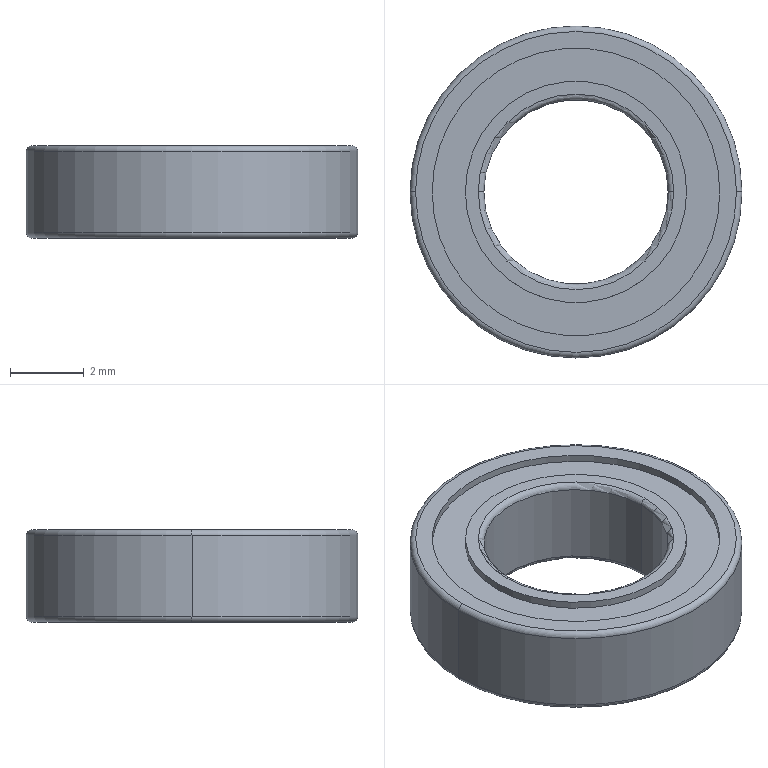Part | NX | features BREP 1 | 1 solid | 26 faces | box 9 x 9 x 2.5 mm | volume 101.727 mm3 | cylinder 12 | torus 8 | plane 6 | commonest cylinder face diameters 6 x4 7.8 x4 5 x2 9 x2
STEP:
#1=CARTESIAN_POINT('',(-4.35,0.,1.25));
#2=VERTEX_POINT('',#1);
#3=CARTESIAN_POINT('',(-4.5,0.,1.1));
#4=VERTEX_POINT('',#3);
#5=CARTESIAN_POINT('',(-4.35,0.,1.1));
#6=DIRECTION('',(0.,1.,0.));
#7=DIRECTION('',(-1.,0.,0.));
#8=AXIS2_PLACEMENT_3D('',#5,#6,#7);
#9=CIRCLE('',#8,0.15);
#10=EDGE_CURVE('',#2,#4,#9,.F.);
#11=ORIENTED_EDGE('',*,*,#10,.T.);
#12=CARTESIAN_POINT('',(4.5,0.,1.1));
#13=VERTEX_POINT('',#12);
#14=CARTESIAN_POINT('',(0.,0.,1.1));
#15=DIRECTION('',(0.,0.,-1.));
#16=DIRECTION('',(1.,0.,0.));
#17=AXIS2_PLACEMENT_3D('',#14,#15,#16);
#18=CIRCLE('',#17,4.5);
#19=EDGE_CURVE('',#13,#4,#18,.T.);
#20=ORIENTED_EDGE('',*,*,#19,.F.);
#21=CARTESIAN_POINT('',(4.35,0.,1.25));
#22=VERTEX_POINT('',#21);
#23=CARTESIAN_POINT('',(4.35,0.,1.1));
#24=DIRECTION('',(0.,-1.,0.));
#25=DIRECTION('',(0.,0.,-1.));
#26=AXIS2_PLACEMENT_3D('',#23,#24,#25);
#27=CIRCLE('',#26,0.15);
#28=EDGE_CURVE('',#22,#13,#27,.F.);
#29=ORIENTED_EDGE('',*,*,#28,.F.);
#30=CARTESIAN_POINT('',(0.,0.,1.25));
#31=DIRECTION('',(0.,0.,1.));
#32=DIRECTION('',(1.,0.,0.));
#33=AXIS2_PLACEMENT_3D('',#30,#31,#32);
#34=CIRCLE('',#33,4.35);
#35=EDGE_CURVE('',#2,#22,#34,.T.);
#36=ORIENTED_EDGE('',*,*,#35,.F.);
#37=EDGE_LOOP('',(#11,#20,#29,#36));
#38=FACE_BOUND('',#37,.T.);
#39=CARTESIAN_POINT('',(0.,0.,1.1));
#40=DIRECTION('',(0.,0.,1.));
#41=DIRECTION('',(1.,0.,0.));
#42=AXIS2_PLACEMENT_3D('',#39,#40,#41);
#43=TOROIDAL_SURFACE('',#42,4.35,0.15);
#44=ADVANCED_FACE('',(#38),#43,.T.);
#45=CARTESIAN_POINT('',(-4.5,0.,-1.1));
#46=VERTEX_POINT('',#45);
#47=CARTESIAN_POINT('',(-4.35,0.,-1.25));
#48=VERTEX_POINT('',#47);
#49=CARTESIAN_POINT('',(-4.35,0.,-1.1));
#50=DIRECTION('',(0.,1.,0.));
#51=DIRECTION('',(-1.,0.,0.));
#52=AXIS2_PLACEMENT_3D('',#49,#50,#51);
#53=CIRCLE('',#52,0.15);
#54=EDGE_CURVE('',#46,#48,#53,.F.);
#55=ORIENTED_EDGE('',*,*,#54,.T.);
#56=CARTESIAN_POINT('',(4.35,0.,-1.25));
#57=VERTEX_POINT('',#56);
#58=CARTESIAN_POINT('',(0.,0.,-1.25));
#59=DIRECTION('',(0.,0.,-1.));
#60=DIRECTION('',(1.,0.,0.));
#61=AXIS2_PLACEMENT_3D('',#58,#59,#60);
#62=CIRCLE('',#61,4.35);
#63=EDGE_CURVE('',#57,#48,#62,.T.);
#64=ORIENTED_EDGE('',*,*,#63,.F.);
#65=CARTESIAN_POINT('',(4.5,0.,-1.1));
#66=VERTEX_POINT('',#65);
#67=CARTESIAN_POINT('',(4.35,0.,-1.1));
#68=DIRECTION('',(0.,-1.,0.));
#69=DIRECTION('',(0.,0.,-1.));
#70=AXIS2_PLACEMENT_3D('',#67,#68,#69);
#71=CIRCLE('',#70,0.15);
#72=EDGE_CURVE('',#66,#57,#71,.F.);
#73=ORIENTED_EDGE('',*,*,#72,.F.);
#74=CARTESIAN_POINT('',(0.,0.,-1.1));
#75=DIRECTION('',(0.,0.,1.));
#76=DIRECTION('',(1.,0.,0.));
#77=AXIS2_PLACEMENT_3D('',#74,#75,#76);
#78=CIRCLE('',#77,4.5);
#79=EDGE_CURVE('',#46,#66,#78,.T.);
#80=ORIENTED_EDGE('',*,*,#79,.F.);
#81=EDGE_LOOP('',(#55,#64,#73,#80));
#82=FACE_BOUND('',#81,.T.);
#83=CARTESIAN_POINT('',(0.,0.,-1.1));
#84=DIRECTION('',(0.,0.,1.));
#85=DIRECTION('',(1.,0.,0.));
#86=AXIS2_PLACEMENT_3D('',#83,#84,#85);
#87=TOROIDAL_SURFACE('',#86,4.35,0.15);
#88=ADVANCED_FACE('',(#82),#87,.T.);
#89=CARTESIAN_POINT('',(-2.5,0.,1.1));
#90=VERTEX_POINT('',#89);
#91=CARTESIAN_POINT('',(-2.65,0.,1.25));
#92=VERTEX_POINT('',#91);
#93=CARTESIAN_POINT('',(-2.65,0.,1.1));
#94=DIRECTION('',(0.,1.,0.));
#95=DIRECTION('',(-1.,0.,0.));
#96=AXIS2_PLACEMENT_3D('',#93,#94,#95);
#97=CIRCLE('',#96,0.15);
#98=EDGE_CURVE('',#90,#92,#97,.F.);
#99=ORIENTED_EDGE('',*,*,#98,.T.);
#100=CARTESIAN_POINT('',(2.65,0.,1.25));
#101=VERTEX_POINT('',#100);
#102=CARTESIAN_POINT('',(0.,0.,1.25));
#103=DIRECTION('',(0.,0.,-1.));
#104=DIRECTION('',(1.,0.,0.));
#105=AXIS2_PLACEMENT_3D('',#102,#103,#104);
#106=CIRCLE('',#105,2.65);
#107=EDGE_CURVE('',#101,#92,#106,.T.);
#108=ORIENTED_EDGE('',*,*,#107,.F.);
#109=CARTESIAN_POINT('',(2.5,0.,1.1));
#110=VERTEX_POINT('',#109);
#111=CARTESIAN_POINT('',(2.65,0.,1.1));
#112=DIRECTION('',(0.,-1.,0.));
#113=DIRECTION('',(0.,0.,-1.));
#114=AXIS2_PLACEMENT_3D('',#111,#112,#113);
#115=CIRCLE('',#114,0.15);
#116=EDGE_CURVE('',#110,#101,#115,.F.);
#117=ORIENTED_EDGE('',*,*,#116,.F.);
#118=CARTESIAN_POINT('',(0.,0.,1.1));
#119=DIRECTION('',(0.,0.,1.));
#120=DIRECTION('',(1.,0.,0.));
#121=AXIS2_PLACEMENT_3D('',#118,#119,#120);
#122=CIRCLE('',#121,2.5);
#123=EDGE_CURVE('',#90,#110,#122,.T.);
#124=ORIENTED_EDGE('',*,*,#123,.F.);
#125=EDGE_LOOP('',(#99,#108,#117,#124));
#126=FACE_BOUND('',#125,.T.);
#127=CARTESIAN_POINT('',(0.,0.,1.1));
#128=DIRECTION('',(0.,0.,1.));
#129=DIRECTION('',(1.,0.,0.));
#130=AXIS2_PLACEMENT_3D('',#127,#128,#129);
#131=TOROIDAL_SURFACE('',#130,2.65,0.15);
#132=ADVANCED_FACE('',(#126),#131,.T.);
#133=CARTESIAN_POINT('',(-2.65,0.,-1.25));
#134=VERTEX_POINT('',#133);
#135=CARTESIAN_POINT('',(-2.5,0.,-1.1));
#136=VERTEX_POINT('',#135);
#137=CARTESIAN_POINT('',(-2.65,0.,-1.1));
#138=DIRECTION('',(0.,1.,0.));
#139=DIRECTION('',(-1.,0.,0.));
#140=AXIS2_PLACEMENT_3D('',#137,#138,#139);
#141=CIRCLE('',#140,0.15);
#142=EDGE_CURVE('',#134,#136,#141,.F.);
#143=ORIENTED_EDGE('',*,*,#142,.T.);
#144=CARTESIAN_POINT('',(2.5,0.,-1.1));
#145=VERTEX_POINT('',#144);
#146=CARTESIAN_POINT('',(0.,0.,-1.1));
#147=DIRECTION('',(0.,0.,-1.));
#148=DIRECTION('',(1.,0.,0.));
#149=AXIS2_PLACEMENT_3D('',#146,#147,#148);
#150=CIRCLE('',#149,2.5);
#151=EDGE_CURVE('',#145,#136,#150,.T.);
#152=ORIENTED_EDGE('',*,*,#151,.F.);
#153=CARTESIAN_POINT('',(2.65,0.,-1.25));
#154=VERTEX_POINT('',#153);
#155=CARTESIAN_POINT('',(2.65,0.,-1.1));
#156=DIRECTION('',(0.,-1.,0.));
#157=DIRECTION('',(0.,0.,-1.));
#158=AXIS2_PLACEMENT_3D('',#155,#156,#157);
#159=CIRCLE('',#158,0.15);
#160=EDGE_CURVE('',#154,#145,#159,.F.);
#161=ORIENTED_EDGE('',*,*,#160,.F.);
#162=CARTESIAN_POINT('',(0.,0.,-1.25));
#163=DIRECTION('',(0.,0.,1.));
#164=DIRECTION('',(1.,0.,0.));
#165=AXIS2_PLACEMENT_3D('',#162,#163,#164);
#166=CIRCLE('',#165,2.65);
#167=EDGE_CURVE('',#134,#154,#166,.T.);
#168=ORIENTED_EDGE('',*,*,#167,.F.);
#169=EDGE_LOOP('',(#143,#152,#161,#168));
#170=FACE_BOUND('',#169,.T.);
#171=CARTESIAN_POINT('',(0.,0.,-1.1));
#172=DIRECTION('',(0.,0.,1.));
#173=DIRECTION('',(1.,0.,0.));
#174=AXIS2_PLACEMENT_3D('',#171,#172,#173);
#175=TOROIDAL_SURFACE('',#174,2.65,0.15);
#176=ADVANCED_FACE('',(#170),#175,.T.);
#177=CARTESIAN_POINT('',(3.,0.,-1.05));
#178=VERTEX_POINT('',#177);
#179=CARTESIAN_POINT('',(3.,0.,-1.25));
#180=VERTEX_POINT('',#179);
#181=CARTESIAN_POINT('',(3.,0.,-1.05));
#182=DIRECTION('',(0.,0.,-1.));
#183=VECTOR('',#182,1000.);
#184=LINE('',#181,#183);
#185=EDGE_CURVE('',#178,#180,#184,.T.);
#186=ORIENTED_EDGE('',*,*,#185,.F.);
#187=CARTESIAN_POINT('',(-3.,0.,-1.05));
#188=VERTEX_POINT('',#187);
#189=CARTESIAN_POINT('',(0.,0.,-1.05));
#190=DIRECTION('',(0.,0.,1.));
#191=DIRECTION('',(1.,0.,0.));
#192=AXIS2_PLACEMENT_3D('',#189,#190,#191);
#193=CIRCLE('',#192,3.);
#194=EDGE_CURVE('',#188,#178,#193,.T.);
#195=ORIENTED_EDGE('',*,*,#194,.F.);
#196=CARTESIAN_POINT('',(-3.,0.,-1.25));
#197=VERTEX_POINT('',#196);
#198=CARTESIAN_POINT('',(-3.,0.,-1.05));
#199=DIRECTION('',(0.,0.,-1.));
#200=VECTOR('',#199,1000.);
#201=LINE('',#198,#200);
#202=EDGE_CURVE('',#188,#197,#201,.T.);
#203=ORIENTED_EDGE('',*,*,#202,.T.);
#204=CARTESIAN_POINT('',(0.,0.,-1.25));
#205=DIRECTION('',(0.,0.,1.));
#206=DIRECTION('',(1.,0.,0.));
#207=AXIS2_PLACEMENT_3D('',#204,#205,#206);
#208=CIRCLE('',#207,3.);
#209=EDGE_CURVE('',#197,#180,#208,.T.);
#210=ORIENTED_EDGE('',*,*,#209,.T.);
#211=EDGE_LOOP('',(#186,#195,#203,#210));
#212=FACE_BOUND('',#211,.T.);
#213=CARTESIAN_POINT('',(0.,0.,-1.05));
#214=DIRECTION('',(0.,0.,-1.));
#215=DIRECTION('',(-1.,0.,0.));
#216=AXIS2_PLACEMENT_3D('',#213,#214,#215);
#217=CYLINDRICAL_SURFACE('',#216,3.);
#218=ADVANCED_FACE('',(#212),#217,.T.);
#219=CARTESIAN_POINT('',(3.9,0.,-1.05));
#220=VERTEX_POINT('',#219);
#221=CARTESIAN_POINT('',(3.9,0.,-1.25));
#222=VERTEX_POINT('',#221);
#223=CARTESIAN_POINT('',(3.9,0.,-1.05));
#224=DIRECTION('',(0.,0.,-1.));
#225=VECTOR('',#224,1000.);
#226=LINE('',#223,#225);
#227=EDGE_CURVE('',#220,#222,#226,.T.);
#228=ORIENTED_EDGE('',*,*,#227,.F.);
#229=CARTESIAN_POINT('',(-3.9,0.,-1.05));
#230=VERTEX_POINT('',#229);
#231=CARTESIAN_POINT('',(0.,0.,-1.05));
#232=DIRECTION('',(0.,0.,1.));
#233=DIRECTION('',(1.,0.,0.));
#234=AXIS2_PLACEMENT_3D('',#231,#232,#233);
#235=CIRCLE('',#234,3.9);
#236=EDGE_CURVE('',#220,#230,#235,.T.);
#237=ORIENTED_EDGE('',*,*,#236,.T.);
#238=CARTESIAN_POINT('',(-3.9,0.,-1.25));
#239=VERTEX_POINT('',#238);
#240=CARTESIAN_POINT('',(-3.9,0.,-1.05));
#241=DIRECTION('',(0.,0.,-1.));
#242=VECTOR('',#241,1000.);
#243=LINE('',#240,#242);
#244=EDGE_CURVE('',#230,#239,#243,.T.);
#245=ORIENTED_EDGE('',*,*,#244,.T.);
#246=CARTESIAN_POINT('',(0.,0.,-1.25));
#247=DIRECTION('',(0.,0.,1.));
#248=DIRECTION('',(1.,0.,0.));
#249=AXIS2_PLACEMENT_3D('',#246,#247,#248);
#250=CIRCLE('',#249,3.9);
#251=EDGE_CURVE('',#222,#239,#250,.T.);
#252=ORIENTED_EDGE('',*,*,#251,.F.);
#253=EDGE_LOOP('',(#228,#237,#245,#252));
#254=FACE_BOUND('',#253,.T.);
#255=CARTESIAN_POINT('',(0.,0.,-1.05));
#256=DIRECTION('',(0.,0.,-1.));
#257=DIRECTION('',(-1.,0.,0.));
#258=AXIS2_PLACEMENT_3D('',#255,#256,#257);
#259=CYLINDRICAL_SURFACE('',#258,3.9);
#260=ADVANCED_FACE('',(#254),#259,.F.);
#261=ORIENTED_EDGE('',*,*,#194,.T.);
#262=CARTESIAN_POINT('',(0.,0.,-1.05));
#263=DIRECTION('',(0.,0.,1.));
#264=DIRECTION('',(1.,0.,0.));
#265=AXIS2_PLACEMENT_3D('',#262,#263,#264);
#266=CIRCLE('',#265,3.);
#267=EDGE_CURVE('',#178,#188,#266,.T.);
#268=ORIENTED_EDGE('',*,*,#267,.T.);
#269=EDGE_LOOP('',(#261,#268));
#270=FACE_BOUND('',#269,.T.);
#271=CARTESIAN_POINT('',(0.,0.,-1.05));
#272=DIRECTION('',(0.,0.,1.));
#273=DIRECTION('',(1.,0.,0.));
#274=AXIS2_PLACEMENT_3D('',#271,#272,#273);
#275=CIRCLE('',#274,3.9);
#276=EDGE_CURVE('',#230,#220,#275,.T.);
#277=ORIENTED_EDGE('',*,*,#276,.F.);
#278=ORIENTED_EDGE('',*,*,#236,.F.);
#279=EDGE_LOOP('',(#277,#278));
#280=FACE_BOUND('',#279,.T.);
#281=CARTESIAN_POINT('',(0.,0.,-1.05));
#282=DIRECTION('',(0.,0.,-1.));
#283=DIRECTION('',(1.,0.,0.));
#284=AXIS2_PLACEMENT_3D('',#281,#282,#283);
#285=PLANE('',#284);
#286=ADVANCED_FACE('',(#270,#280),#285,.T.);
#287=CARTESIAN_POINT('',(-3.,0.,1.25));
#288=VERTEX_POINT('',#287);
#289=CARTESIAN_POINT('',(-3.,0.,1.05));
#290=VERTEX_POINT('',#289);
#291=CARTESIAN_POINT('',(-3.,0.,1.05));
#292=DIRECTION('',(0.,0.,1.));
#293=VECTOR('',#292,1000.);
#294=LINE('',#291,#293);
#295=EDGE_CURVE('',#288,#290,#294,.F.);
#296=ORIENTED_EDGE('',*,*,#295,.T.);
#297=CARTESIAN_POINT('',(3.,0.,1.05));
#298=VERTEX_POINT('',#297);
#299=CARTESIAN_POINT('',(0.,0.,1.05));
#300=DIRECTION('',(0.,0.,1.));
#301=DIRECTION('',(1.,0.,0.));
#302=AXIS2_PLACEMENT_3D('',#299,#300,#301);
#303=CIRCLE('',#302,3.);
#304=EDGE_CURVE('',#290,#298,#303,.T.);
#305=ORIENTED_EDGE('',*,*,#304,.T.);
#306=CARTESIAN_POINT('',(3.,0.,1.25));
#307=VERTEX_POINT('',#306);
#308=CARTESIAN_POINT('',(3.,0.,1.05));
#309=DIRECTION('',(0.,0.,1.));
#310=VECTOR('',#309,1000.);
#311=LINE('',#308,#310);
#312=EDGE_CURVE('',#307,#298,#311,.F.);
#313=ORIENTED_EDGE('',*,*,#312,.F.);
#314=CARTESIAN_POINT('',(0.,0.,1.25));
#315=DIRECTION('',(0.,0.,1.));
#316=DIRECTION('',(1.,0.,0.));
#317=AXIS2_PLACEMENT_3D('',#314,#315,#316);
#318=CIRCLE('',#317,3.);
#319=EDGE_CURVE('',#288,#307,#318,.T.);
#320=ORIENTED_EDGE('',*,*,#319,.F.);
#321=EDGE_LOOP('',(#296,#305,#313,#320));
#322=FACE_BOUND('',#321,.T.);
#323=CARTESIAN_POINT('',(0.,0.,1.05));
#324=DIRECTION('',(0.,0.,1.));
#325=DIRECTION('',(1.,0.,0.));
#326=AXIS2_PLACEMENT_3D('',#323,#324,#325);
#327=CYLINDRICAL_SURFACE('',#326,3.);
#328=ADVANCED_FACE('',(#322),#327,.T.);
#329=CARTESIAN_POINT('',(3.9,0.,1.05));
#330=VERTEX_POINT('',#329);
#331=CARTESIAN_POINT('',(-3.9,0.,1.05));
#332=VERTEX_POINT('',#331);
#333=CARTESIAN_POINT('',(0.,0.,1.05));
#334=DIRECTION('',(0.,0.,1.));
#335=DIRECTION('',(1.,0.,0.));
#336=AXIS2_PLACEMENT_3D('',#333,#334,#335);
#337=CIRCLE('',#336,3.9);
#338=EDGE_CURVE('',#330,#332,#337,.T.);
#339=ORIENTED_EDGE('',*,*,#338,.T.);
#340=CARTESIAN_POINT('',(0.,0.,1.05));
#341=DIRECTION('',(0.,0.,1.));
#342=DIRECTION('',(1.,0.,0.));
#343=AXIS2_PLACEMENT_3D('',#340,#341,#342);
#344=CIRCLE('',#343,3.9);
#345=EDGE_CURVE('',#332,#330,#344,.T.);
#346=ORIENTED_EDGE('',*,*,#345,.T.);
#347=EDGE_LOOP('',(#339,#346));
#348=FACE_BOUND('',#347,.T.);
#349=CARTESIAN_POINT('',(0.,0.,1.05));
#350=DIRECTION('',(0.,0.,1.));
#351=DIRECTION('',(1.,0.,0.));
#352=AXIS2_PLACEMENT_3D('',#349,#350,#351);
#353=CIRCLE('',#352,3.);
#354=EDGE_CURVE('',#298,#290,#353,.T.);
#355=ORIENTED_EDGE('',*,*,#354,.F.);
#356=ORIENTED_EDGE('',*,*,#304,.F.);
#357=EDGE_LOOP('',(#355,#356));
#358=FACE_BOUND('',#357,.T.);
#359=CARTESIAN_POINT('',(0.,0.,1.05));
#360=DIRECTION('',(0.,0.,1.));
#361=DIRECTION('',(1.,0.,0.));
#362=AXIS2_PLACEMENT_3D('',#359,#360,#361);
#363=PLANE('',#362);
#364=ADVANCED_FACE('',(#348,#358),#363,.T.);
#365=CARTESIAN_POINT('',(-3.9,0.,1.25));
#366=VERTEX_POINT('',#365);
#367=CARTESIAN_POINT('',(-3.9,0.,1.05));
#368=DIRECTION('',(0.,0.,1.));
#369=VECTOR('',#368,1000.);
#370=LINE('',#367,#369);
#371=EDGE_CURVE('',#366,#332,#370,.F.);
#372=ORIENTED_EDGE('',*,*,#371,.T.);
#373=ORIENTED_EDGE('',*,*,#338,.F.);
#374=CARTESIAN_POINT('',(3.9,0.,1.25));
#375=VERTEX_POINT('',#374);
#376=CARTESIAN_POINT('',(3.9,0.,1.05));
#377=DIRECTION('',(0.,0.,1.));
#378=VECTOR('',#377,1000.);
#379=LINE('',#376,#378);
#380=EDGE_CURVE('',#375,#330,#379,.F.);
#381=ORIENTED_EDGE('',*,*,#380,.F.);
#382=CARTESIAN_POINT('',(0.,0.,1.25));
#383=DIRECTION('',(0.,0.,1.));
#384=DIRECTION('',(1.,0.,0.));
#385=AXIS2_PLACEMENT_3D('',#382,#383,#384);
#386=CIRCLE('',#385,3.9);
#387=EDGE_CURVE('',#375,#366,#386,.T.);
#388=ORIENTED_EDGE('',*,*,#387,.T.);
#389=EDGE_LOOP('',(#372,#373,#381,#388));
#390=FACE_BOUND('',#389,.T.);
#391=CARTESIAN_POINT('',(0.,0.,1.05));
#392=DIRECTION('',(0.,0.,1.));
#393=DIRECTION('',(1.,0.,0.));
#394=AXIS2_PLACEMENT_3D('',#391,#392,#393);
#395=CYLINDRICAL_SURFACE('',#394,3.9);
#396=ADVANCED_FACE('',(#390),#395,.F.);
#397=CARTESIAN_POINT('',(2.5,0.,1.25));
#398=DIRECTION('',(0.,0.,-1.));
#399=VECTOR('',#398,1000.);
#400=LINE('',#397,#399);
#401=EDGE_CURVE('',#110,#145,#400,.T.);
#402=ORIENTED_EDGE('',*,*,#401,.F.);
#403=CARTESIAN_POINT('',(0.,0.,1.1));
#404=DIRECTION('',(0.,0.,1.));
#405=DIRECTION('',(1.,0.,0.));
#406=AXIS2_PLACEMENT_3D('',#403,#404,#405);
#407=CIRCLE('',#406,2.5);
#408=EDGE_CURVE('',#110,#90,#407,.T.);
#409=ORIENTED_EDGE('',*,*,#408,.T.);
#410=CARTESIAN_POINT('',(-2.5,0.,1.25));
#411=DIRECTION('',(0.,0.,-1.));
#412=VECTOR('',#411,1000.);
#413=LINE('',#410,#412);
#414=EDGE_CURVE('',#90,#136,#413,.T.);
#415=ORIENTED_EDGE('',*,*,#414,.T.);
#416=CARTESIAN_POINT('',(0.,0.,-1.1));
#417=DIRECTION('',(0.,0.,-1.));
#418=DIRECTION('',(1.,0.,0.));
#419=AXIS2_PLACEMENT_3D('',#416,#417,#418);
#420=CIRCLE('',#419,2.5);
#421=EDGE_CURVE('',#136,#145,#420,.T.);
#422=ORIENTED_EDGE('',*,*,#421,.T.);
#423=EDGE_LOOP('',(#402,#409,#415,#422));
#424=FACE_BOUND('',#423,.T.);
#425=CARTESIAN_POINT('',(0.,0.,1.25));
#426=DIRECTION('',(0.,0.,-1.));
#427=DIRECTION('',(-1.,0.,0.));
#428=AXIS2_PLACEMENT_3D('',#425,#426,#427);
#429=CYLINDRICAL_SURFACE('',#428,2.5);
#430=ADVANCED_FACE('',(#424),#429,.F.);
#431=CARTESIAN_POINT('',(4.5,0.,1.25));
#432=DIRECTION('',(0.,0.,-1.));
#433=VECTOR('',#432,1000.);
#434=LINE('',#431,#433);
#435=EDGE_CURVE('',#13,#66,#434,.T.);
#436=ORIENTED_EDGE('',*,*,#435,.F.);
#437=ORIENTED_EDGE('',*,*,#19,.T.);
#438=CARTESIAN_POINT('',(-4.5,0.,1.25));
#439=DIRECTION('',(0.,0.,-1.));
#440=VECTOR('',#439,1000.);
#441=LINE('',#438,#440);
#442=EDGE_CURVE('',#4,#46,#441,.T.);
#443=ORIENTED_EDGE('',*,*,#442,.T.);
#444=ORIENTED_EDGE('',*,*,#79,.T.);
#445=EDGE_LOOP('',(#436,#437,#443,#444));
#446=FACE_BOUND('',#445,.T.);
#447=CARTESIAN_POINT('',(0.,0.,1.25));
#448=DIRECTION('',(0.,0.,-1.));
#449=DIRECTION('',(-1.,0.,0.));
#450=AXIS2_PLACEMENT_3D('',#447,#448,#449);
#451=CYLINDRICAL_SURFACE('',#450,4.5);
#452=ADVANCED_FACE('',(#446),#451,.T.);
#453=CARTESIAN_POINT('',(0.,0.,-1.25));
#454=DIRECTION('',(0.,0.,1.));
#455=DIRECTION('',(1.,0.,0.));
#456=AXIS2_PLACEMENT_3D('',#453,#454,#455);
#457=CIRCLE('',#456,3.9);
#458=EDGE_CURVE('',#239,#222,#457,.T.);
#459=ORIENTED_EDGE('',*,*,#458,.T.);
#460=ORIENTED_EDGE('',*,*,#251,.T.);
#461=EDGE_LOOP('',(#459,#460));
#462=FACE_BOUND('',#461,.T.);
#463=ORIENTED_EDGE('',*,*,#63,.T.);
#464=CARTESIAN_POINT('',(0.,0.,-1.25));
#465=DIRECTION('',(0.,0.,-1.));
#466=DIRECTION('',(1.,0.,0.));
#467=AXIS2_PLACEMENT_3D('',#464,#465,#466);
#468=CIRCLE('',#467,4.35);
#469=EDGE_CURVE('',#48,#57,#468,.T.);
#470=ORIENTED_EDGE('',*,*,#469,.T.);
#471=EDGE_LOOP('',(#463,#470));
#472=FACE_BOUND('',#471,.T.);
#473=CARTESIAN_POINT('',(0.,0.,-1.25));
#474=DIRECTION('',(0.,0.,1.));
#475=DIRECTION('',(1.,0.,0.));
#476=AXIS2_PLACEMENT_3D('',#473,#474,#475);
#477=PLANE('',#476);
#478=ADVANCED_FACE('',(#462,#472),#477,.F.);
#479=ORIENTED_EDGE('',*,*,#387,.F.);
#480=CARTESIAN_POINT('',(0.,0.,1.25));
#481=DIRECTION('',(0.,0.,1.));
#482=DIRECTION('',(1.,0.,0.));
#483=AXIS2_PLACEMENT_3D('',#480,#481,#482);
#484=CIRCLE('',#483,3.9);
#485=EDGE_CURVE('',#366,#375,#484,.T.);
#486=ORIENTED_EDGE('',*,*,#485,.F.);
#487=EDGE_LOOP('',(#479,#486));
#488=FACE_BOUND('',#487,.T.);
#489=CARTESIAN_POINT('',(0.,0.,1.25));
#490=DIRECTION('',(0.,0.,1.));
#491=DIRECTION('',(1.,0.,0.));
#492=AXIS2_PLACEMENT_3D('',#489,#490,#491);
#493=CIRCLE('',#492,4.35);
#494=EDGE_CURVE('',#22,#2,#493,.T.);
#495=ORIENTED_EDGE('',*,*,#494,.T.);
#496=ORIENTED_EDGE('',*,*,#35,.T.);
#497=EDGE_LOOP('',(#495,#496));
#498=FACE_BOUND('',#497,.T.);
#499=CARTESIAN_POINT('',(0.,0.,1.25));
#500=DIRECTION('',(0.,0.,1.));
#501=DIRECTION('',(1.,0.,0.));
#502=AXIS2_PLACEMENT_3D('',#499,#500,#501);
#503=PLANE('',#502);
#504=ADVANCED_FACE('',(#488,#498),#503,.T.);
#505=CARTESIAN_POINT('',(0.,0.,1.25));
#506=DIRECTION('',(0.,0.,1.));
#507=DIRECTION('',(1.,0.,0.));
#508=AXIS2_PLACEMENT_3D('',#505,#506,#507);
#509=CIRCLE('',#508,3.);
#510=EDGE_CURVE('',#307,#288,#509,.T.);
#511=ORIENTED_EDGE('',*,*,#510,.T.);
#512=ORIENTED_EDGE('',*,*,#319,.T.);
#513=EDGE_LOOP('',(#511,#512));
#514=FACE_BOUND('',#513,.T.);
#515=ORIENTED_EDGE('',*,*,#107,.T.);
#516=CARTESIAN_POINT('',(0.,0.,1.25));
#517=DIRECTION('',(0.,0.,-1.));
#518=DIRECTION('',(1.,0.,0.));
#519=AXIS2_PLACEMENT_3D('',#516,#517,#518);
#520=CIRCLE('',#519,2.65);
#521=EDGE_CURVE('',#92,#101,#520,.T.);
#522=ORIENTED_EDGE('',*,*,#521,.T.);
#523=EDGE_LOOP('',(#515,#522));
#524=FACE_BOUND('',#523,.T.);
#525=CARTESIAN_POINT('',(0.,0.,1.25));
#526=DIRECTION('',(0.,0.,1.));
#527=DIRECTION('',(1.,0.,0.));
#528=AXIS2_PLACEMENT_3D('',#525,#526,#527);
#529=PLANE('',#528);
#530=ADVANCED_FACE('',(#514,#524),#529,.T.);
#531=ORIENTED_EDGE('',*,*,#209,.F.);
#532=CARTESIAN_POINT('',(0.,0.,-1.25));
#533=DIRECTION('',(0.,0.,1.));
#534=DIRECTION('',(1.,0.,0.));
#535=AXIS2_PLACEMENT_3D('',#532,#533,#534);
#536=CIRCLE('',#535,3.);
#537=EDGE_CURVE('',#180,#197,#536,.T.);
#538=ORIENTED_EDGE('',*,*,#537,.F.);
#539=EDGE_LOOP('',(#531,#538));
#540=FACE_BOUND('',#539,.T.);
#541=CARTESIAN_POINT('',(0.,0.,-1.25));
#542=DIRECTION('',(0.,0.,1.));
#543=DIRECTION('',(1.,0.,0.));
#544=AXIS2_PLACEMENT_3D('',#541,#542,#543);
#545=CIRCLE('',#544,2.65);
#546=EDGE_CURVE('',#154,#134,#545,.T.);
#547=ORIENTED_EDGE('',*,*,#546,.T.);
#548=ORIENTED_EDGE('',*,*,#167,.T.);
#549=EDGE_LOOP('',(#547,#548));
#550=FACE_BOUND('',#549,.T.);
#551=CARTESIAN_POINT('',(0.,0.,-1.25));
#552=DIRECTION('',(0.,0.,1.));
#553=DIRECTION('',(1.,0.,0.));
#554=AXIS2_PLACEMENT_3D('',#551,#552,#553);
#555=PLANE('',#554);
#556=ADVANCED_FACE('',(#540,#550),#555,.F.);
#557=CARTESIAN_POINT('',(0.,0.,1.1));
#558=DIRECTION('',(0.,0.,-1.));
#559=DIRECTION('',(1.,0.,0.));
#560=AXIS2_PLACEMENT_3D('',#557,#558,#559);
#561=CIRCLE('',#560,4.5);
#562=EDGE_CURVE('',#4,#13,#561,.T.);
#563=ORIENTED_EDGE('',*,*,#562,.T.);
#564=ORIENTED_EDGE('',*,*,#435,.T.);
#565=CARTESIAN_POINT('',(0.,0.,-1.1));
#566=DIRECTION('',(0.,0.,1.));
#567=DIRECTION('',(1.,0.,0.));
#568=AXIS2_PLACEMENT_3D('',#565,#566,#567);
#569=CIRCLE('',#568,4.5);
#570=EDGE_CURVE('',#66,#46,#569,.T.);
#571=ORIENTED_EDGE('',*,*,#570,.T.);
#572=ORIENTED_EDGE('',*,*,#442,.F.);
#573=EDGE_LOOP('',(#563,#564,#571,#572));
#574=FACE_BOUND('',#573,.T.);
#575=CARTESIAN_POINT('',(0.,0.,1.25));
#576=DIRECTION('',(0.,0.,-1.));
#577=DIRECTION('',(-1.,0.,0.));
#578=AXIS2_PLACEMENT_3D('',#575,#576,#577);
#579=CYLINDRICAL_SURFACE('',#578,4.5);
#580=ADVANCED_FACE('',(#574),#579,.T.);
#581=ORIENTED_EDGE('',*,*,#123,.T.);
#582=ORIENTED_EDGE('',*,*,#401,.T.);
#583=ORIENTED_EDGE('',*,*,#151,.T.);
#584=ORIENTED_EDGE('',*,*,#414,.F.);
#585=EDGE_LOOP('',(#581,#582,#583,#584));
#586=FACE_BOUND('',#585,.T.);
#587=CARTESIAN_POINT('',(0.,0.,1.25));
#588=DIRECTION('',(0.,0.,-1.));
#589=DIRECTION('',(-1.,0.,0.));
#590=AXIS2_PLACEMENT_3D('',#587,#588,#589);
#591=CYLINDRICAL_SURFACE('',#590,2.5);
#592=ADVANCED_FACE('',(#586),#591,.F.);
#593=ORIENTED_EDGE('',*,*,#345,.F.);
#594=ORIENTED_EDGE('',*,*,#371,.F.);
#595=ORIENTED_EDGE('',*,*,#485,.T.);
#596=ORIENTED_EDGE('',*,*,#380,.T.);
#597=EDGE_LOOP('',(#593,#594,#595,#596));
#598=FACE_BOUND('',#597,.T.);
#599=CARTESIAN_POINT('',(0.,0.,1.05));
#600=DIRECTION('',(0.,0.,1.));
#601=DIRECTION('',(1.,0.,0.));
#602=AXIS2_PLACEMENT_3D('',#599,#600,#601);
#603=CYLINDRICAL_SURFACE('',#602,3.9);
#604=ADVANCED_FACE('',(#598),#603,.F.);
#605=ORIENTED_EDGE('',*,*,#354,.T.);
#606=ORIENTED_EDGE('',*,*,#295,.F.);
#607=ORIENTED_EDGE('',*,*,#510,.F.);
#608=ORIENTED_EDGE('',*,*,#312,.T.);
#609=EDGE_LOOP('',(#605,#606,#607,#608));
#610=FACE_BOUND('',#609,.T.);
#611=CARTESIAN_POINT('',(0.,0.,1.05));
#612=DIRECTION('',(0.,0.,1.));
#613=DIRECTION('',(1.,0.,0.));
#614=AXIS2_PLACEMENT_3D('',#611,#612,#613);
#615=CYLINDRICAL_SURFACE('',#614,3.);
#616=ADVANCED_FACE('',(#610),#615,.T.);
#617=ORIENTED_EDGE('',*,*,#276,.T.);
#618=ORIENTED_EDGE('',*,*,#227,.T.);
#619=ORIENTED_EDGE('',*,*,#458,.F.);
#620=ORIENTED_EDGE('',*,*,#244,.F.);
#621=EDGE_LOOP('',(#617,#618,#619,#620));
#622=FACE_BOUND('',#621,.T.);
#623=CARTESIAN_POINT('',(0.,0.,-1.05));
#624=DIRECTION('',(0.,0.,-1.));
#625=DIRECTION('',(-1.,0.,0.));
#626=AXIS2_PLACEMENT_3D('',#623,#624,#625);
#627=CYLINDRICAL_SURFACE('',#626,3.9);
#628=ADVANCED_FACE('',(#622),#627,.F.);
#629=ORIENTED_EDGE('',*,*,#267,.F.);
#630=ORIENTED_EDGE('',*,*,#185,.T.);
#631=ORIENTED_EDGE('',*,*,#537,.T.);
#632=ORIENTED_EDGE('',*,*,#202,.F.);
#633=EDGE_LOOP('',(#629,#630,#631,#632));
#634=FACE_BOUND('',#633,.T.);
#635=CARTESIAN_POINT('',(0.,0.,-1.05));
#636=DIRECTION('',(0.,0.,-1.));
#637=DIRECTION('',(-1.,0.,0.));
#638=AXIS2_PLACEMENT_3D('',#635,#636,#637);
#639=CYLINDRICAL_SURFACE('',#638,3.);
#640=ADVANCED_FACE('',(#634),#639,.T.);
#641=ORIENTED_EDGE('',*,*,#421,.F.);
#642=ORIENTED_EDGE('',*,*,#142,.F.);
#643=ORIENTED_EDGE('',*,*,#546,.F.);
#644=ORIENTED_EDGE('',*,*,#160,.T.);
#645=EDGE_LOOP('',(#641,#642,#643,#644));
#646=FACE_BOUND('',#645,.T.);
#647=CARTESIAN_POINT('',(0.,0.,-1.1));
#648=DIRECTION('',(0.,0.,1.));
#649=DIRECTION('',(1.,0.,0.));
#650=AXIS2_PLACEMENT_3D('',#647,#648,#649);
#651=TOROIDAL_SURFACE('',#650,2.65,0.15);
#652=ADVANCED_FACE('',(#646),#651,.T.);
#653=ORIENTED_EDGE('',*,*,#521,.F.);
#654=ORIENTED_EDGE('',*,*,#98,.F.);
#655=ORIENTED_EDGE('',*,*,#408,.F.);
#656=ORIENTED_EDGE('',*,*,#116,.T.);
#657=EDGE_LOOP('',(#653,#654,#655,#656));
#658=FACE_BOUND('',#657,.T.);
#659=CARTESIAN_POINT('',(0.,0.,1.1));
#660=DIRECTION('',(0.,0.,1.));
#661=DIRECTION('',(1.,0.,0.));
#662=AXIS2_PLACEMENT_3D('',#659,#660,#661);
#663=TOROIDAL_SURFACE('',#662,2.65,0.15);
#664=ADVANCED_FACE('',(#658),#663,.T.);
#665=ORIENTED_EDGE('',*,*,#469,.F.);
#666=ORIENTED_EDGE('',*,*,#54,.F.);
#667=ORIENTED_EDGE('',*,*,#570,.F.);
#668=ORIENTED_EDGE('',*,*,#72,.T.);
#669=EDGE_LOOP('',(#665,#666,#667,#668));
#670=FACE_BOUND('',#669,.T.);
#671=CARTESIAN_POINT('',(0.,0.,-1.1));
#672=DIRECTION('',(0.,0.,1.));
#673=DIRECTION('',(1.,0.,0.));
#674=AXIS2_PLACEMENT_3D('',#671,#672,#673);
#675=TOROIDAL_SURFACE('',#674,4.35,0.15);
#676=ADVANCED_FACE('',(#670),#675,.T.);
#677=ORIENTED_EDGE('',*,*,#562,.F.);
#678=ORIENTED_EDGE('',*,*,#10,.F.);
#679=ORIENTED_EDGE('',*,*,#494,.F.);
#680=ORIENTED_EDGE('',*,*,#28,.T.);
#681=EDGE_LOOP('',(#677,#678,#679,#680));
#682=FACE_BOUND('',#681,.T.);
#683=CARTESIAN_POINT('',(0.,0.,1.1));
#684=DIRECTION('',(0.,0.,1.));
#685=DIRECTION('',(1.,0.,0.));
#686=AXIS2_PLACEMENT_3D('',#683,#684,#685);
#687=TOROIDAL_SURFACE('',#686,4.35,0.15);
#688=ADVANCED_FACE('',(#682),#687,.T.);
#689=CLOSED_SHELL('',(#44,#88,#132,#176,#218,#260,#286,#328,#364,#396,#430,#452,#478,#504,#530,#556,#580,#592,#604,#616,#628,#640,#652,#664,#676,#688));
#690=MANIFOLD_SOLID_BREP('',#689);
#691=(LENGTH_UNIT()NAMED_UNIT(*)SI_UNIT(.MILLI.,.METRE.));
#692=UNCERTAINTY_MEASURE_WITH_UNIT(LENGTH_MEASURE(0.00001),#691,'','');
#693=(NAMED_UNIT(*)PLANE_ANGLE_UNIT()SI_UNIT($,.RADIAN.));
#694=(NAMED_UNIT(*)SI_UNIT($,.STERADIAN.)SOLID_ANGLE_UNIT());
#695=(GEOMETRIC_REPRESENTATION_CONTEXT(3)GLOBAL_UNCERTAINTY_ASSIGNED_CONTEXT((#692))GLOBAL_UNIT_ASSIGNED_CONTEXT((#691,#693,#694))REPRESENTATION_CONTEXT('',''));
#696=ADVANCED_BREP_SHAPE_REPRESENTATION('',(#690),#695);